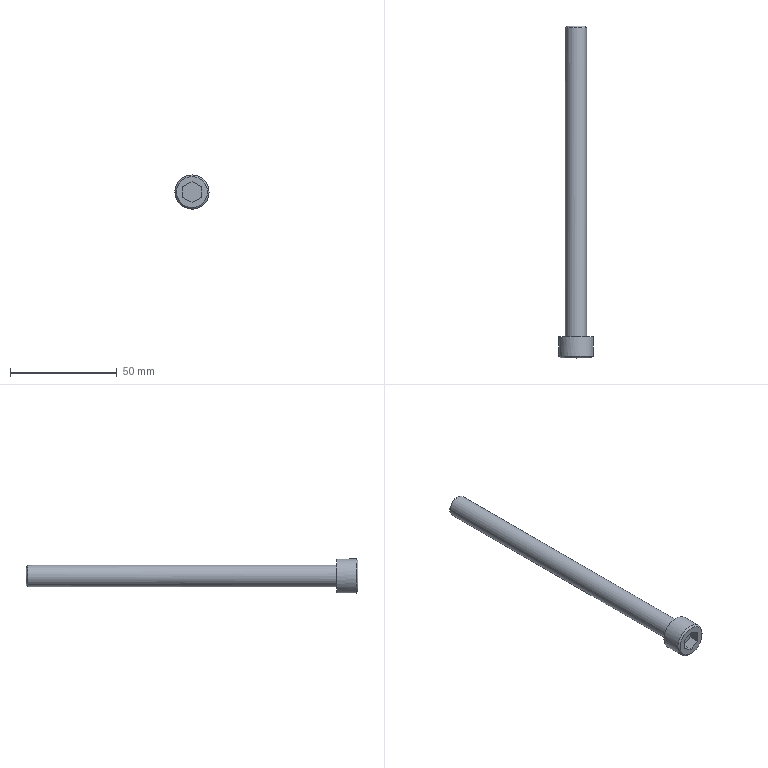Part | NX | features M10.00-155.00 2 | 1 solid | 14 faces | box 16 x 155.5 x 16 mm | volume 13103 mm3 | plane 10 | cylinder 2 | cone 2 | commonest cylinder face diameters 10 x1 16 x1
STEP:
#1=CARTESIAN_POINT('',(-41.,-290.5,-55.75));
#2=VERTEX_POINT('',#1);
#3=CARTESIAN_POINT('',(-41.,-290.5,-63.));
#4=DIRECTION('',(0.,1.,0.));
#5=DIRECTION('',(0.,0.,1.));
#6=AXIS2_PLACEMENT_3D('',#3,#4,#5);
#7=CIRCLE('',#6,7.25);
#8=EDGE_CURVE('',#2,#2,#7,.T.);
#9=ORIENTED_EDGE('',*,*,#8,.F.);
#10=EDGE_LOOP('',(#9));
#11=FACE_BOUND('',#10,.T.);
#12=CARTESIAN_POINT('',(-45.25,-290.5,-65.454));
#13=VERTEX_POINT('',#12);
#14=CARTESIAN_POINT('',(-45.25,-290.5,-60.546));
#15=VERTEX_POINT('',#14);
#16=CARTESIAN_POINT('',(-45.25,-290.5,-65.454));
#17=DIRECTION('',(0.,0.,1.));
#18=VECTOR('',#17,1000.);
#19=LINE('',#16,#18);
#20=EDGE_CURVE('',#13,#15,#19,.T.);
#21=ORIENTED_EDGE('',*,*,#20,.T.);
#22=CARTESIAN_POINT('',(-41.,-290.5,-58.093));
#23=VERTEX_POINT('',#22);
#24=CARTESIAN_POINT('',(-45.25,-290.5,-60.546));
#25=DIRECTION('',(0.866,0.,0.5));
#26=VECTOR('',#25,1000.);
#27=LINE('',#24,#26);
#28=EDGE_CURVE('',#15,#23,#27,.T.);
#29=ORIENTED_EDGE('',*,*,#28,.T.);
#30=CARTESIAN_POINT('',(-36.75,-290.5,-60.546));
#31=VERTEX_POINT('',#30);
#32=CARTESIAN_POINT('',(-41.,-290.5,-58.093));
#33=DIRECTION('',(0.866,0.,-0.5));
#34=VECTOR('',#33,1000.);
#35=LINE('',#32,#34);
#36=EDGE_CURVE('',#23,#31,#35,.T.);
#37=ORIENTED_EDGE('',*,*,#36,.T.);
#38=CARTESIAN_POINT('',(-36.75,-290.5,-65.454));
#39=VERTEX_POINT('',#38);
#40=CARTESIAN_POINT('',(-36.75,-290.5,-60.546));
#41=DIRECTION('',(0.,0.,-1.));
#42=VECTOR('',#41,1000.);
#43=LINE('',#40,#42);
#44=EDGE_CURVE('',#31,#39,#43,.T.);
#45=ORIENTED_EDGE('',*,*,#44,.T.);
#46=CARTESIAN_POINT('',(-41.,-290.5,-67.907));
#47=VERTEX_POINT('',#46);
#48=CARTESIAN_POINT('',(-36.75,-290.5,-65.454));
#49=DIRECTION('',(-0.866,0.,-0.5));
#50=VECTOR('',#49,1000.);
#51=LINE('',#48,#50);
#52=EDGE_CURVE('',#39,#47,#51,.T.);
#53=ORIENTED_EDGE('',*,*,#52,.T.);
#54=CARTESIAN_POINT('',(-41.,-290.5,-67.907));
#55=DIRECTION('',(-0.866,0.,0.5));
#56=VECTOR('',#55,1000.);
#57=LINE('',#54,#56);
#58=EDGE_CURVE('',#47,#13,#57,.T.);
#59=ORIENTED_EDGE('',*,*,#58,.T.);
#60=EDGE_LOOP('',(#21,#29,#37,#45,#53,#59));
#61=FACE_BOUND('',#60,.T.);
#62=CARTESIAN_POINT('',(-41.,-290.5,-63.));
#63=DIRECTION('',(0.,-1.,0.));
#64=DIRECTION('',(0.,0.,1.));
#65=AXIS2_PLACEMENT_3D('',#62,#63,#64);
#66=PLANE('',#65);
#67=ADVANCED_FACE('',(#11,#61),#66,.T.);
#68=CARTESIAN_POINT('',(-36.,-280.5,-63.));
#69=VERTEX_POINT('',#68);
#70=CARTESIAN_POINT('',(-41.,-280.5,-63.));
#71=DIRECTION('',(0.,-1.,0.));
#72=DIRECTION('',(1.,0.,0.));
#73=AXIS2_PLACEMENT_3D('',#70,#71,#72);
#74=CIRCLE('',#73,5.);
#75=EDGE_CURVE('',#69,#69,#74,.T.);
#76=ORIENTED_EDGE('',*,*,#75,.T.);
#77=EDGE_LOOP('',(#76));
#78=FACE_BOUND('',#77,.T.);
#79=CARTESIAN_POINT('',(-33.,-280.5,-63.));
#80=VERTEX_POINT('',#79);
#81=CARTESIAN_POINT('',(-41.,-280.5,-63.));
#82=DIRECTION('',(0.,1.,0.));
#83=DIRECTION('',(1.,0.,0.));
#84=AXIS2_PLACEMENT_3D('',#81,#82,#83);
#85=CIRCLE('',#84,8.);
#86=EDGE_CURVE('',#80,#80,#85,.T.);
#87=ORIENTED_EDGE('',*,*,#86,.T.);
#88=EDGE_LOOP('',(#87));
#89=FACE_BOUND('',#88,.T.);
#90=CARTESIAN_POINT('',(-41.,-280.5,-63.));
#91=DIRECTION('',(0.,1.,0.));
#92=DIRECTION('',(0.,0.,-1.));
#93=AXIS2_PLACEMENT_3D('',#90,#91,#92);
#94=PLANE('',#93);
#95=ADVANCED_FACE('',(#78,#89),#94,.T.);
#96=CARTESIAN_POINT('',(-41.,-289.75,-55.));
#97=VERTEX_POINT('',#96);
#98=CARTESIAN_POINT('',(-41.,-289.75,-63.));
#99=DIRECTION('',(0.,1.,0.));
#100=DIRECTION('',(0.,0.,1.));
#101=AXIS2_PLACEMENT_3D('',#98,#99,#100);
#102=CIRCLE('',#101,8.);
#103=EDGE_CURVE('',#97,#97,#102,.F.);
#104=ORIENTED_EDGE('',*,*,#103,.F.);
#105=EDGE_LOOP('',(#104));
#106=FACE_BOUND('',#105,.T.);
#107=ORIENTED_EDGE('',*,*,#86,.F.);
#108=EDGE_LOOP('',(#107));
#109=FACE_BOUND('',#108,.T.);
#110=CARTESIAN_POINT('',(-41.,-280.5,-63.));
#111=DIRECTION('',(0.,-1.,0.));
#112=DIRECTION('',(1.,0.,0.));
#113=AXIS2_PLACEMENT_3D('',#110,#111,#112);
#114=CYLINDRICAL_SURFACE('',#113,8.);
#115=ADVANCED_FACE('',(#106,#109),#114,.T.);
#116=CARTESIAN_POINT('',(-41.,-135.,-67.25));
#117=VERTEX_POINT('',#116);
#118=CARTESIAN_POINT('',(-41.,-135.,-63.));
#119=DIRECTION('',(0.,-1.,0.));
#120=DIRECTION('',(0.,0.,-1.));
#121=AXIS2_PLACEMENT_3D('',#118,#119,#120);
#122=CIRCLE('',#121,4.25);
#123=EDGE_CURVE('',#117,#117,#122,.T.);
#124=ORIENTED_EDGE('',*,*,#123,.F.);
#125=EDGE_LOOP('',(#124));
#126=FACE_BOUND('',#125,.T.);
#127=CARTESIAN_POINT('',(-41.,-135.,-63.));
#128=DIRECTION('',(0.,1.,0.));
#129=DIRECTION('',(0.,0.,-1.));
#130=AXIS2_PLACEMENT_3D('',#127,#128,#129);
#131=PLANE('',#130);
#132=ADVANCED_FACE('',(#126),#131,.T.);
#133=CARTESIAN_POINT('',(-41.,-135.75,-68.));
#134=VERTEX_POINT('',#133);
#135=CARTESIAN_POINT('',(-41.,-135.75,-63.));
#136=DIRECTION('',(0.,-1.,0.));
#137=DIRECTION('',(0.,0.,-1.));
#138=AXIS2_PLACEMENT_3D('',#135,#136,#137);
#139=CIRCLE('',#138,5.);
#140=EDGE_CURVE('',#134,#134,#139,.F.);
#141=ORIENTED_EDGE('',*,*,#140,.F.);
#142=EDGE_LOOP('',(#141));
#143=FACE_BOUND('',#142,.T.);
#144=ORIENTED_EDGE('',*,*,#75,.F.);
#145=EDGE_LOOP('',(#144));
#146=FACE_BOUND('',#145,.T.);
#147=CARTESIAN_POINT('',(-41.,-280.5,-63.));
#148=DIRECTION('',(0.,1.,0.));
#149=DIRECTION('',(1.,0.,0.));
#150=AXIS2_PLACEMENT_3D('',#147,#148,#149);
#151=CYLINDRICAL_SURFACE('',#150,5.);
#152=ADVANCED_FACE('',(#143,#146),#151,.T.);
#153=ORIENTED_EDGE('',*,*,#28,.F.);
#154=CARTESIAN_POINT('',(-45.25,-285.5,-60.546));
#155=VERTEX_POINT('',#154);
#156=CARTESIAN_POINT('',(-45.25,-285.5,-60.546));
#157=DIRECTION('',(0.,-1.,0.));
#158=VECTOR('',#157,1000.);
#159=LINE('',#156,#158);
#160=EDGE_CURVE('',#15,#155,#159,.F.);
#161=ORIENTED_EDGE('',*,*,#160,.T.);
#162=CARTESIAN_POINT('',(-41.,-285.5,-58.093));
#163=VERTEX_POINT('',#162);
#164=CARTESIAN_POINT('',(-45.25,-285.5,-60.546));
#165=DIRECTION('',(0.866,0.,0.5));
#166=VECTOR('',#165,1000.);
#167=LINE('',#164,#166);
#168=EDGE_CURVE('',#163,#155,#167,.F.);
#169=ORIENTED_EDGE('',*,*,#168,.F.);
#170=CARTESIAN_POINT('',(-41.,-285.5,-58.093));
#171=DIRECTION('',(0.,-1.,0.));
#172=VECTOR('',#171,1000.);
#173=LINE('',#170,#172);
#174=EDGE_CURVE('',#23,#163,#173,.F.);
#175=ORIENTED_EDGE('',*,*,#174,.F.);
#176=EDGE_LOOP('',(#153,#161,#169,#175));
#177=FACE_BOUND('',#176,.T.);
#178=CARTESIAN_POINT('',(-43.125,-288.,-59.319));
#179=DIRECTION('',(-0.5,0.,0.866));
#180=DIRECTION('',(0.866,0.,0.5));
#181=AXIS2_PLACEMENT_3D('',#178,#179,#180);
#182=PLANE('',#181);
#183=ADVANCED_FACE('',(#177),#182,.F.);
#184=ORIENTED_EDGE('',*,*,#20,.F.);
#185=CARTESIAN_POINT('',(-45.25,-285.5,-65.454));
#186=VERTEX_POINT('',#185);
#187=CARTESIAN_POINT('',(-45.25,-285.5,-65.454));
#188=DIRECTION('',(0.,-1.,0.));
#189=VECTOR('',#188,1000.);
#190=LINE('',#187,#189);
#191=EDGE_CURVE('',#13,#186,#190,.F.);
#192=ORIENTED_EDGE('',*,*,#191,.T.);
#193=CARTESIAN_POINT('',(-45.25,-285.5,-65.454));
#194=DIRECTION('',(0.,0.,1.));
#195=VECTOR('',#194,1000.);
#196=LINE('',#193,#195);
#197=EDGE_CURVE('',#155,#186,#196,.F.);
#198=ORIENTED_EDGE('',*,*,#197,.F.);
#199=ORIENTED_EDGE('',*,*,#160,.F.);
#200=EDGE_LOOP('',(#184,#192,#198,#199));
#201=FACE_BOUND('',#200,.T.);
#202=CARTESIAN_POINT('',(-45.25,-288.,-63.));
#203=DIRECTION('',(-1.,0.,0.));
#204=DIRECTION('',(0.,1.,0.));
#205=AXIS2_PLACEMENT_3D('',#202,#203,#204);
#206=PLANE('',#205);
#207=ADVANCED_FACE('',(#201),#206,.F.);
#208=ORIENTED_EDGE('',*,*,#58,.F.);
#209=CARTESIAN_POINT('',(-41.,-285.5,-67.907));
#210=VERTEX_POINT('',#209);
#211=CARTESIAN_POINT('',(-41.,-285.5,-67.907));
#212=DIRECTION('',(0.,-1.,0.));
#213=VECTOR('',#212,1000.);
#214=LINE('',#211,#213);
#215=EDGE_CURVE('',#47,#210,#214,.F.);
#216=ORIENTED_EDGE('',*,*,#215,.T.);
#217=CARTESIAN_POINT('',(-41.,-285.5,-67.907));
#218=DIRECTION('',(-0.866,0.,0.5));
#219=VECTOR('',#218,1000.);
#220=LINE('',#217,#219);
#221=EDGE_CURVE('',#186,#210,#220,.F.);
#222=ORIENTED_EDGE('',*,*,#221,.F.);
#223=ORIENTED_EDGE('',*,*,#191,.F.);
#224=EDGE_LOOP('',(#208,#216,#222,#223));
#225=FACE_BOUND('',#224,.T.);
#226=CARTESIAN_POINT('',(-43.125,-288.,-66.681));
#227=DIRECTION('',(-0.5,0.,-0.866));
#228=DIRECTION('',(-0.866,0.,0.5));
#229=AXIS2_PLACEMENT_3D('',#226,#227,#228);
#230=PLANE('',#229);
#231=ADVANCED_FACE('',(#225),#230,.F.);
#232=ORIENTED_EDGE('',*,*,#52,.F.);
#233=CARTESIAN_POINT('',(-36.75,-285.5,-65.454));
#234=VERTEX_POINT('',#233);
#235=CARTESIAN_POINT('',(-36.75,-285.5,-65.454));
#236=DIRECTION('',(0.,-1.,0.));
#237=VECTOR('',#236,1000.);
#238=LINE('',#235,#237);
#239=EDGE_CURVE('',#39,#234,#238,.F.);
#240=ORIENTED_EDGE('',*,*,#239,.T.);
#241=CARTESIAN_POINT('',(-36.75,-285.5,-65.454));
#242=DIRECTION('',(-0.866,0.,-0.5));
#243=VECTOR('',#242,1000.);
#244=LINE('',#241,#243);
#245=EDGE_CURVE('',#210,#234,#244,.F.);
#246=ORIENTED_EDGE('',*,*,#245,.F.);
#247=ORIENTED_EDGE('',*,*,#215,.F.);
#248=EDGE_LOOP('',(#232,#240,#246,#247));
#249=FACE_BOUND('',#248,.T.);
#250=CARTESIAN_POINT('',(-38.875,-288.,-66.681));
#251=DIRECTION('',(0.5,0.,-0.866));
#252=DIRECTION('',(-0.866,0.,-0.5));
#253=AXIS2_PLACEMENT_3D('',#250,#251,#252);
#254=PLANE('',#253);
#255=ADVANCED_FACE('',(#249),#254,.F.);
#256=ORIENTED_EDGE('',*,*,#44,.F.);
#257=CARTESIAN_POINT('',(-36.75,-285.5,-60.546));
#258=VERTEX_POINT('',#257);
#259=CARTESIAN_POINT('',(-36.75,-285.5,-60.546));
#260=DIRECTION('',(0.,-1.,0.));
#261=VECTOR('',#260,1000.);
#262=LINE('',#259,#261);
#263=EDGE_CURVE('',#31,#258,#262,.F.);
#264=ORIENTED_EDGE('',*,*,#263,.T.);
#265=CARTESIAN_POINT('',(-36.75,-285.5,-60.546));
#266=DIRECTION('',(0.,0.,-1.));
#267=VECTOR('',#266,1000.);
#268=LINE('',#265,#267);
#269=EDGE_CURVE('',#234,#258,#268,.F.);
#270=ORIENTED_EDGE('',*,*,#269,.F.);
#271=ORIENTED_EDGE('',*,*,#239,.F.);
#272=EDGE_LOOP('',(#256,#264,#270,#271));
#273=FACE_BOUND('',#272,.T.);
#274=CARTESIAN_POINT('',(-36.75,-288.,-63.));
#275=DIRECTION('',(1.,0.,0.));
#276=DIRECTION('',(0.,-1.,0.));
#277=AXIS2_PLACEMENT_3D('',#274,#275,#276);
#278=PLANE('',#277);
#279=ADVANCED_FACE('',(#273),#278,.F.);
#280=ORIENTED_EDGE('',*,*,#36,.F.);
#281=ORIENTED_EDGE('',*,*,#174,.T.);
#282=CARTESIAN_POINT('',(-41.,-285.5,-58.093));
#283=DIRECTION('',(0.866,0.,-0.5));
#284=VECTOR('',#283,1000.);
#285=LINE('',#282,#284);
#286=EDGE_CURVE('',#258,#163,#285,.F.);
#287=ORIENTED_EDGE('',*,*,#286,.F.);
#288=ORIENTED_EDGE('',*,*,#263,.F.);
#289=EDGE_LOOP('',(#280,#281,#287,#288));
#290=FACE_BOUND('',#289,.T.);
#291=CARTESIAN_POINT('',(-38.875,-288.,-59.319));
#292=DIRECTION('',(0.5,0.,0.866));
#293=DIRECTION('',(0.866,0.,-0.5));
#294=AXIS2_PLACEMENT_3D('',#291,#292,#293);
#295=PLANE('',#294);
#296=ADVANCED_FACE('',(#290),#295,.F.);
#297=ORIENTED_EDGE('',*,*,#286,.T.);
#298=ORIENTED_EDGE('',*,*,#168,.T.);
#299=ORIENTED_EDGE('',*,*,#197,.T.);
#300=ORIENTED_EDGE('',*,*,#221,.T.);
#301=ORIENTED_EDGE('',*,*,#245,.T.);
#302=ORIENTED_EDGE('',*,*,#269,.T.);
#303=EDGE_LOOP('',(#297,#298,#299,#300,#301,#302));
#304=FACE_BOUND('',#303,.T.);
#305=CARTESIAN_POINT('',(-41.,-285.5,-63.));
#306=DIRECTION('',(0.,1.,0.));
#307=DIRECTION('',(0.,0.,-1.));
#308=AXIS2_PLACEMENT_3D('',#305,#306,#307);
#309=PLANE('',#308);
#310=ADVANCED_FACE('',(#304),#309,.F.);
#311=ORIENTED_EDGE('',*,*,#123,.T.);
#312=EDGE_LOOP('',(#311));
#313=FACE_BOUND('',#312,.T.);
#314=ORIENTED_EDGE('',*,*,#140,.T.);
#315=EDGE_LOOP('',(#314));
#316=FACE_BOUND('',#315,.T.);
#317=CARTESIAN_POINT('',(-41.,-135.75,-63.));
#318=DIRECTION('',(0.,-1.,0.));
#319=DIRECTION('',(0.,0.,1.));
#320=AXIS2_PLACEMENT_3D('',#317,#318,#319);
#321=CONICAL_SURFACE('',#320,5.,0.7854);
#322=ADVANCED_FACE('',(#313,#316),#321,.T.);
#323=ORIENTED_EDGE('',*,*,#8,.T.);
#324=EDGE_LOOP('',(#323));
#325=FACE_BOUND('',#324,.T.);
#326=ORIENTED_EDGE('',*,*,#103,.T.);
#327=EDGE_LOOP('',(#326));
#328=FACE_BOUND('',#327,.T.);
#329=CARTESIAN_POINT('',(-41.,-289.75,-63.));
#330=DIRECTION('',(0.,1.,0.));
#331=DIRECTION('',(0.,0.,-1.));
#332=AXIS2_PLACEMENT_3D('',#329,#330,#331);
#333=CONICAL_SURFACE('',#332,8.,0.7854);
#334=ADVANCED_FACE('',(#325,#328),#333,.T.);
#335=CLOSED_SHELL('',(#67,#95,#115,#132,#152,#183,#207,#231,#255,#279,#296,#310,#322,#334));
#336=MANIFOLD_SOLID_BREP('',#335);
#337=(LENGTH_UNIT()NAMED_UNIT(*)SI_UNIT(.MILLI.,.METRE.));
#338=UNCERTAINTY_MEASURE_WITH_UNIT(LENGTH_MEASURE(0.00001),#337,'','');
#339=(NAMED_UNIT(*)PLANE_ANGLE_UNIT()SI_UNIT($,.RADIAN.));
#340=(NAMED_UNIT(*)SI_UNIT($,.STERADIAN.)SOLID_ANGLE_UNIT());
#341=(GEOMETRIC_REPRESENTATION_CONTEXT(3)GLOBAL_UNCERTAINTY_ASSIGNED_CONTEXT((#338))GLOBAL_UNIT_ASSIGNED_CONTEXT((#337,#339,#340))REPRESENTATION_CONTEXT('',''));
#342=ADVANCED_BREP_SHAPE_REPRESENTATION('',(#336),#341);